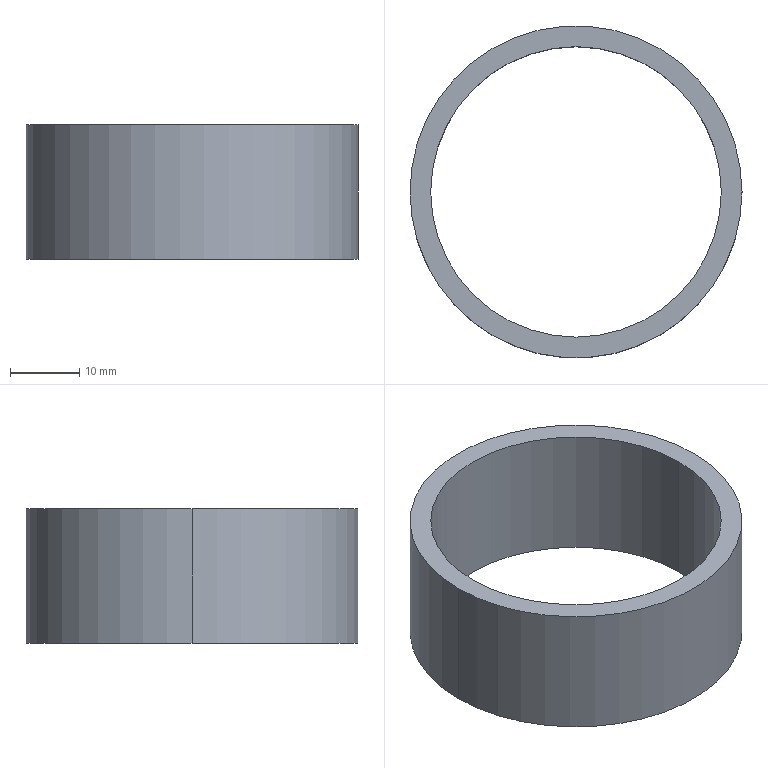Part | STEP file | 04-Spacer 1 | 1 solid | 6 faces | box 48 x 48 x 19.5 mm | volume 8270 mm3 | cylinder 4 | plane 2 | commonest cylinder face diameters 42 x2 48 x2
STEP:
#1=CARTESIAN_POINT('',(0.,0.,0.));
#2=DIRECTION('',(0.,0.,1.));
#3=DIRECTION('',(1.,0.,0.));
#4=AXIS2_PLACEMENT_3D('',#1,#2,#3);
#5=CARTESIAN_POINT('',(-21.,0.,19.5));
#6=VERTEX_POINT('',#5);
#7=CARTESIAN_POINT('',(-21.,0.,0.));
#8=VERTEX_POINT('',#7);
#9=CARTESIAN_POINT('',(-21.,0.,19.5));
#10=DIRECTION('',(0.,0.,-1.));
#11=VECTOR('',#10,1.);
#12=LINE('',#9,#11);
#13=CARTESIAN_POINT('',(0.,0.,19.5));
#14=DIRECTION('',(0.,0.,-1.));
#15=DIRECTION('',(-1.,0.,0.));
#16=AXIS2_PLACEMENT_3D('',#13,#14,#15);
#17=CYLINDRICAL_SURFACE('',#16,21.);
#18=CARTESIAN_POINT('',(6.283,0.));
#19=DIRECTION('',(0.,1.));
#20=VECTOR('',#19,1.);
#21=LINE('',#18,#20);
#22=(GEOMETRIC_REPRESENTATION_CONTEXT(2)PARAMETRIC_REPRESENTATION_CONTEXT()REPRESENTATION_CONTEXT('',''));
#23=DEFINITIONAL_REPRESENTATION('',(#21),#22);
#24=PCURVE('',#17,#23);
#25=CARTESIAN_POINT('',(0.,0.,19.5));
#26=DIRECTION('',(0.,0.,-1.));
#27=DIRECTION('',(-1.,0.,0.));
#28=AXIS2_PLACEMENT_3D('',#25,#26,#27);
#29=CYLINDRICAL_SURFACE('',#28,21.);
#30=CARTESIAN_POINT('',(0.,0.));
#31=DIRECTION('',(0.,1.));
#32=VECTOR('',#31,1.);
#33=LINE('',#30,#32);
#34=(GEOMETRIC_REPRESENTATION_CONTEXT(2)PARAMETRIC_REPRESENTATION_CONTEXT()REPRESENTATION_CONTEXT('',''));
#35=DEFINITIONAL_REPRESENTATION('',(#33),#34);
#36=PCURVE('',#29,#35);
#37=SURFACE_CURVE('',#12,(#24,#36),.PCURVE_S1.);
#38=EDGE_CURVE('',#6,#8,#37,.T.);
#39=ORIENTED_EDGE('',*,*,#38,.T.);
#40=CARTESIAN_POINT('',(21.,0.,0.));
#41=VERTEX_POINT('',#40);
#42=CARTESIAN_POINT('',(0.,0.,0.));
#43=DIRECTION('',(0.,0.,1.));
#44=DIRECTION('',(1.,0.,0.));
#45=AXIS2_PLACEMENT_3D('',#42,#43,#44);
#46=CIRCLE('',#45,21.);
#47=CARTESIAN_POINT('',(9.425,19.5));
#48=DIRECTION('',(-1.,0.));
#49=VECTOR('',#48,1.);
#50=LINE('',#47,#49);
#51=(GEOMETRIC_REPRESENTATION_CONTEXT(2)PARAMETRIC_REPRESENTATION_CONTEXT()REPRESENTATION_CONTEXT('',''));
#52=DEFINITIONAL_REPRESENTATION('',(#50),#51);
#53=PCURVE('',#17,#52);
#54=CARTESIAN_POINT('',(0.,0.,0.));
#55=DIRECTION('',(0.,0.,1.));
#56=DIRECTION('',(1.,0.,0.));
#57=AXIS2_PLACEMENT_3D('',#54,#55,#56);
#58=PLANE('',#57);
#59=CARTESIAN_POINT('',(0.,0.));
#60=DIRECTION('',(1.,0.));
#61=AXIS2_PLACEMENT_2D('',#59,#60);
#62=CIRCLE('',#61,21.);
#63=(GEOMETRIC_REPRESENTATION_CONTEXT(2)PARAMETRIC_REPRESENTATION_CONTEXT()REPRESENTATION_CONTEXT('',''));
#64=DEFINITIONAL_REPRESENTATION('',(#62),#63);
#65=PCURVE('',#58,#64);
#66=SURFACE_CURVE('',#46,(#53,#65),.PCURVE_S1.);
#67=EDGE_CURVE('',#8,#41,#66,.T.);
#68=ORIENTED_EDGE('',*,*,#67,.T.);
#69=CARTESIAN_POINT('',(21.,0.,19.5));
#70=VERTEX_POINT('',#69);
#71=CARTESIAN_POINT('',(21.,0.,19.5));
#72=DIRECTION('',(0.,0.,-1.));
#73=VECTOR('',#72,1.);
#74=LINE('',#71,#73);
#75=CARTESIAN_POINT('',(3.142,0.));
#76=DIRECTION('',(0.,1.));
#77=VECTOR('',#76,1.);
#78=LINE('',#75,#77);
#79=(GEOMETRIC_REPRESENTATION_CONTEXT(2)PARAMETRIC_REPRESENTATION_CONTEXT()REPRESENTATION_CONTEXT('',''));
#80=DEFINITIONAL_REPRESENTATION('',(#78),#79);
#81=PCURVE('',#17,#80);
#82=CARTESIAN_POINT('',(3.142,0.));
#83=DIRECTION('',(0.,1.));
#84=VECTOR('',#83,1.);
#85=LINE('',#82,#84);
#86=(GEOMETRIC_REPRESENTATION_CONTEXT(2)PARAMETRIC_REPRESENTATION_CONTEXT()REPRESENTATION_CONTEXT('',''));
#87=DEFINITIONAL_REPRESENTATION('',(#85),#86);
#88=PCURVE('',#29,#87);
#89=SURFACE_CURVE('',#74,(#81,#88),.PCURVE_S1.);
#90=EDGE_CURVE('',#70,#41,#89,.T.);
#91=ORIENTED_EDGE('',*,*,#90,.F.);
#92=CARTESIAN_POINT('',(0.,0.,19.5));
#93=DIRECTION('',(0.,0.,1.));
#94=DIRECTION('',(1.,0.,0.));
#95=AXIS2_PLACEMENT_3D('',#92,#93,#94);
#96=CIRCLE('',#95,21.);
#97=CARTESIAN_POINT('',(9.425,0.));
#98=DIRECTION('',(-1.,0.));
#99=VECTOR('',#98,1.);
#100=LINE('',#97,#99);
#101=(GEOMETRIC_REPRESENTATION_CONTEXT(2)PARAMETRIC_REPRESENTATION_CONTEXT()REPRESENTATION_CONTEXT('',''));
#102=DEFINITIONAL_REPRESENTATION('',(#100),#101);
#103=PCURVE('',#17,#102);
#104=CARTESIAN_POINT('',(0.,0.,19.5));
#105=DIRECTION('',(0.,0.,1.));
#106=DIRECTION('',(1.,0.,0.));
#107=AXIS2_PLACEMENT_3D('',#104,#105,#106);
#108=PLANE('',#107);
#109=CARTESIAN_POINT('',(0.,0.));
#110=DIRECTION('',(1.,0.));
#111=AXIS2_PLACEMENT_2D('',#109,#110);
#112=CIRCLE('',#111,21.);
#113=(GEOMETRIC_REPRESENTATION_CONTEXT(2)PARAMETRIC_REPRESENTATION_CONTEXT()REPRESENTATION_CONTEXT('',''));
#114=DEFINITIONAL_REPRESENTATION('',(#112),#113);
#115=PCURVE('',#108,#114);
#116=SURFACE_CURVE('',#96,(#103,#115),.PCURVE_S1.);
#117=EDGE_CURVE('',#6,#70,#116,.T.);
#118=ORIENTED_EDGE('',*,*,#117,.F.);
#119=EDGE_LOOP('',(#39,#68,#91,#118));
#120=FACE_BOUND('',#119,.F.);
#121=ADVANCED_FACE('',(#120),#17,.F.);
#122=CARTESIAN_POINT('',(24.,0.,19.5));
#123=VERTEX_POINT('',#122);
#124=CARTESIAN_POINT('',(-24.,0.,19.5));
#125=VERTEX_POINT('',#124);
#126=CARTESIAN_POINT('',(0.,0.,19.5));
#127=DIRECTION('',(0.,0.,1.));
#128=DIRECTION('',(1.,0.,0.));
#129=AXIS2_PLACEMENT_3D('',#126,#127,#128);
#130=CIRCLE('',#129,24.);
#131=CARTESIAN_POINT('',(0.,0.,19.5));
#132=DIRECTION('',(0.,0.,-1.));
#133=DIRECTION('',(-1.,0.,0.));
#134=AXIS2_PLACEMENT_3D('',#131,#132,#133);
#135=CYLINDRICAL_SURFACE('',#134,24.);
#136=CARTESIAN_POINT('',(3.142,0.));
#137=DIRECTION('',(-1.,0.));
#138=VECTOR('',#137,1.);
#139=LINE('',#136,#138);
#140=(GEOMETRIC_REPRESENTATION_CONTEXT(2)PARAMETRIC_REPRESENTATION_CONTEXT()REPRESENTATION_CONTEXT('',''));
#141=DEFINITIONAL_REPRESENTATION('',(#139),#140);
#142=PCURVE('',#135,#141);
#143=CARTESIAN_POINT('',(0.,0.));
#144=DIRECTION('',(1.,0.));
#145=AXIS2_PLACEMENT_2D('',#143,#144);
#146=CIRCLE('',#145,24.);
#147=(GEOMETRIC_REPRESENTATION_CONTEXT(2)PARAMETRIC_REPRESENTATION_CONTEXT()REPRESENTATION_CONTEXT('',''));
#148=DEFINITIONAL_REPRESENTATION('',(#146),#147);
#149=PCURVE('',#108,#148);
#150=SURFACE_CURVE('',#130,(#142,#149),.PCURVE_S1.);
#151=EDGE_CURVE('',#123,#125,#150,.T.);
#152=ORIENTED_EDGE('',*,*,#151,.F.);
#153=CARTESIAN_POINT('',(24.,0.,0.));
#154=VERTEX_POINT('',#153);
#155=CARTESIAN_POINT('',(24.,0.,19.5));
#156=DIRECTION('',(0.,0.,-1.));
#157=VECTOR('',#156,1.);
#158=LINE('',#155,#157);
#159=CARTESIAN_POINT('',(3.142,0.));
#160=DIRECTION('',(0.,1.));
#161=VECTOR('',#160,1.);
#162=LINE('',#159,#161);
#163=(GEOMETRIC_REPRESENTATION_CONTEXT(2)PARAMETRIC_REPRESENTATION_CONTEXT()REPRESENTATION_CONTEXT('',''));
#164=DEFINITIONAL_REPRESENTATION('',(#162),#163);
#165=PCURVE('',#135,#164);
#166=CARTESIAN_POINT('',(0.,0.,19.5));
#167=DIRECTION('',(0.,0.,-1.));
#168=DIRECTION('',(-1.,0.,0.));
#169=AXIS2_PLACEMENT_3D('',#166,#167,#168);
#170=CYLINDRICAL_SURFACE('',#169,24.);
#171=CARTESIAN_POINT('',(3.142,0.));
#172=DIRECTION('',(0.,1.));
#173=VECTOR('',#172,1.);
#174=LINE('',#171,#173);
#175=(GEOMETRIC_REPRESENTATION_CONTEXT(2)PARAMETRIC_REPRESENTATION_CONTEXT()REPRESENTATION_CONTEXT('',''));
#176=DEFINITIONAL_REPRESENTATION('',(#174),#175);
#177=PCURVE('',#170,#176);
#178=SURFACE_CURVE('',#158,(#165,#177),.PCURVE_S1.);
#179=EDGE_CURVE('',#123,#154,#178,.T.);
#180=ORIENTED_EDGE('',*,*,#179,.T.);
#181=CARTESIAN_POINT('',(-24.,0.,0.));
#182=VERTEX_POINT('',#181);
#183=CARTESIAN_POINT('',(0.,0.,0.));
#184=DIRECTION('',(0.,0.,1.));
#185=DIRECTION('',(1.,0.,0.));
#186=AXIS2_PLACEMENT_3D('',#183,#184,#185);
#187=CIRCLE('',#186,24.);
#188=CARTESIAN_POINT('',(3.142,19.5));
#189=DIRECTION('',(-1.,0.));
#190=VECTOR('',#189,1.);
#191=LINE('',#188,#190);
#192=(GEOMETRIC_REPRESENTATION_CONTEXT(2)PARAMETRIC_REPRESENTATION_CONTEXT()REPRESENTATION_CONTEXT('',''));
#193=DEFINITIONAL_REPRESENTATION('',(#191),#192);
#194=PCURVE('',#135,#193);
#195=CARTESIAN_POINT('',(0.,0.));
#196=DIRECTION('',(1.,0.));
#197=AXIS2_PLACEMENT_2D('',#195,#196);
#198=CIRCLE('',#197,24.);
#199=(GEOMETRIC_REPRESENTATION_CONTEXT(2)PARAMETRIC_REPRESENTATION_CONTEXT()REPRESENTATION_CONTEXT('',''));
#200=DEFINITIONAL_REPRESENTATION('',(#198),#199);
#201=PCURVE('',#58,#200);
#202=SURFACE_CURVE('',#187,(#194,#201),.PCURVE_S1.);
#203=EDGE_CURVE('',#154,#182,#202,.T.);
#204=ORIENTED_EDGE('',*,*,#203,.T.);
#205=CARTESIAN_POINT('',(-24.,0.,19.5));
#206=DIRECTION('',(0.,0.,-1.));
#207=VECTOR('',#206,1.);
#208=LINE('',#205,#207);
#209=CARTESIAN_POINT('',(0.,0.));
#210=DIRECTION('',(0.,1.));
#211=VECTOR('',#210,1.);
#212=LINE('',#209,#211);
#213=(GEOMETRIC_REPRESENTATION_CONTEXT(2)PARAMETRIC_REPRESENTATION_CONTEXT()REPRESENTATION_CONTEXT('',''));
#214=DEFINITIONAL_REPRESENTATION('',(#212),#213);
#215=PCURVE('',#135,#214);
#216=CARTESIAN_POINT('',(6.283,0.));
#217=DIRECTION('',(0.,1.));
#218=VECTOR('',#217,1.);
#219=LINE('',#216,#218);
#220=(GEOMETRIC_REPRESENTATION_CONTEXT(2)PARAMETRIC_REPRESENTATION_CONTEXT()REPRESENTATION_CONTEXT('',''));
#221=DEFINITIONAL_REPRESENTATION('',(#219),#220);
#222=PCURVE('',#170,#221);
#223=SURFACE_CURVE('',#208,(#215,#222),.PCURVE_S1.);
#224=EDGE_CURVE('',#125,#182,#223,.T.);
#225=ORIENTED_EDGE('',*,*,#224,.F.);
#226=EDGE_LOOP('',(#152,#180,#204,#225));
#227=FACE_BOUND('',#226,.T.);
#228=ADVANCED_FACE('',(#227),#135,.T.);
#229=CARTESIAN_POINT('',(0.,0.,19.5));
#230=DIRECTION('',(0.,0.,1.));
#231=DIRECTION('',(1.,0.,0.));
#232=AXIS2_PLACEMENT_3D('',#229,#230,#231);
#233=CIRCLE('',#232,24.);
#234=CARTESIAN_POINT('',(0.,0.));
#235=DIRECTION('',(1.,0.));
#236=AXIS2_PLACEMENT_2D('',#234,#235);
#237=CIRCLE('',#236,24.);
#238=(GEOMETRIC_REPRESENTATION_CONTEXT(2)PARAMETRIC_REPRESENTATION_CONTEXT()REPRESENTATION_CONTEXT('',''));
#239=DEFINITIONAL_REPRESENTATION('',(#237),#238);
#240=PCURVE('',#108,#239);
#241=CARTESIAN_POINT('',(9.425,0.));
#242=DIRECTION('',(-1.,0.));
#243=VECTOR('',#242,1.);
#244=LINE('',#241,#243);
#245=(GEOMETRIC_REPRESENTATION_CONTEXT(2)PARAMETRIC_REPRESENTATION_CONTEXT()REPRESENTATION_CONTEXT('',''));
#246=DEFINITIONAL_REPRESENTATION('',(#244),#245);
#247=PCURVE('',#170,#246);
#248=SURFACE_CURVE('',#233,(#240,#247),.PCURVE_S1.);
#249=EDGE_CURVE('',#125,#123,#248,.T.);
#250=ORIENTED_EDGE('',*,*,#249,.T.);
#251=ORIENTED_EDGE('',*,*,#151,.T.);
#252=EDGE_LOOP('',(#250,#251));
#253=FACE_BOUND('',#252,.T.);
#254=ORIENTED_EDGE('',*,*,#117,.F.);
#255=CARTESIAN_POINT('',(0.,0.,19.5));
#256=DIRECTION('',(0.,0.,1.));
#257=DIRECTION('',(1.,0.,0.));
#258=AXIS2_PLACEMENT_3D('',#255,#256,#257);
#259=CIRCLE('',#258,21.);
#260=CARTESIAN_POINT('',(0.,0.));
#261=DIRECTION('',(1.,0.));
#262=AXIS2_PLACEMENT_2D('',#260,#261);
#263=CIRCLE('',#262,21.);
#264=(GEOMETRIC_REPRESENTATION_CONTEXT(2)PARAMETRIC_REPRESENTATION_CONTEXT()REPRESENTATION_CONTEXT('',''));
#265=DEFINITIONAL_REPRESENTATION('',(#263),#264);
#266=PCURVE('',#108,#265);
#267=CARTESIAN_POINT('',(3.142,0.));
#268=DIRECTION('',(-1.,0.));
#269=VECTOR('',#268,1.);
#270=LINE('',#267,#269);
#271=(GEOMETRIC_REPRESENTATION_CONTEXT(2)PARAMETRIC_REPRESENTATION_CONTEXT()REPRESENTATION_CONTEXT('',''));
#272=DEFINITIONAL_REPRESENTATION('',(#270),#271);
#273=PCURVE('',#29,#272);
#274=SURFACE_CURVE('',#259,(#266,#273),.PCURVE_S1.);
#275=EDGE_CURVE('',#70,#6,#274,.T.);
#276=ORIENTED_EDGE('',*,*,#275,.F.);
#277=EDGE_LOOP('',(#254,#276));
#278=FACE_BOUND('',#277,.T.);
#279=ADVANCED_FACE('',(#253,#278),#108,.T.);
#280=CARTESIAN_POINT('',(0.,0.,0.));
#281=DIRECTION('',(0.,0.,1.));
#282=DIRECTION('',(1.,0.,0.));
#283=AXIS2_PLACEMENT_3D('',#280,#281,#282);
#284=CIRCLE('',#283,24.);
#285=CARTESIAN_POINT('',(0.,0.));
#286=DIRECTION('',(1.,0.));
#287=AXIS2_PLACEMENT_2D('',#285,#286);
#288=CIRCLE('',#287,24.);
#289=(GEOMETRIC_REPRESENTATION_CONTEXT(2)PARAMETRIC_REPRESENTATION_CONTEXT()REPRESENTATION_CONTEXT('',''));
#290=DEFINITIONAL_REPRESENTATION('',(#288),#289);
#291=PCURVE('',#58,#290);
#292=CARTESIAN_POINT('',(9.425,19.5));
#293=DIRECTION('',(-1.,0.));
#294=VECTOR('',#293,1.);
#295=LINE('',#292,#294);
#296=(GEOMETRIC_REPRESENTATION_CONTEXT(2)PARAMETRIC_REPRESENTATION_CONTEXT()REPRESENTATION_CONTEXT('',''));
#297=DEFINITIONAL_REPRESENTATION('',(#295),#296);
#298=PCURVE('',#170,#297);
#299=SURFACE_CURVE('',#284,(#291,#298),.PCURVE_S1.);
#300=EDGE_CURVE('',#182,#154,#299,.T.);
#301=ORIENTED_EDGE('',*,*,#300,.F.);
#302=ORIENTED_EDGE('',*,*,#203,.F.);
#303=EDGE_LOOP('',(#301,#302));
#304=FACE_BOUND('',#303,.T.);
#305=ORIENTED_EDGE('',*,*,#67,.T.);
#306=CARTESIAN_POINT('',(0.,0.,0.));
#307=DIRECTION('',(0.,0.,1.));
#308=DIRECTION('',(1.,0.,0.));
#309=AXIS2_PLACEMENT_3D('',#306,#307,#308);
#310=CIRCLE('',#309,21.);
#311=CARTESIAN_POINT('',(0.,0.));
#312=DIRECTION('',(1.,0.));
#313=AXIS2_PLACEMENT_2D('',#311,#312);
#314=CIRCLE('',#313,21.);
#315=(GEOMETRIC_REPRESENTATION_CONTEXT(2)PARAMETRIC_REPRESENTATION_CONTEXT()REPRESENTATION_CONTEXT('',''));
#316=DEFINITIONAL_REPRESENTATION('',(#314),#315);
#317=PCURVE('',#58,#316);
#318=CARTESIAN_POINT('',(3.142,19.5));
#319=DIRECTION('',(-1.,0.));
#320=VECTOR('',#319,1.);
#321=LINE('',#318,#320);
#322=(GEOMETRIC_REPRESENTATION_CONTEXT(2)PARAMETRIC_REPRESENTATION_CONTEXT()REPRESENTATION_CONTEXT('',''));
#323=DEFINITIONAL_REPRESENTATION('',(#321),#322);
#324=PCURVE('',#29,#323);
#325=SURFACE_CURVE('',#310,(#317,#324),.PCURVE_S1.);
#326=EDGE_CURVE('',#41,#8,#325,.T.);
#327=ORIENTED_EDGE('',*,*,#326,.T.);
#328=EDGE_LOOP('',(#305,#327));
#329=FACE_BOUND('',#328,.T.);
#330=ADVANCED_FACE('',(#304,#329),#58,.F.);
#331=ORIENTED_EDGE('',*,*,#179,.F.);
#332=ORIENTED_EDGE('',*,*,#249,.F.);
#333=ORIENTED_EDGE('',*,*,#224,.T.);
#334=ORIENTED_EDGE('',*,*,#300,.T.);
#335=EDGE_LOOP('',(#331,#332,#333,#334));
#336=FACE_BOUND('',#335,.T.);
#337=ADVANCED_FACE('',(#336),#170,.T.);
#338=ORIENTED_EDGE('',*,*,#326,.T.);
#339=ORIENTED_EDGE('',*,*,#38,.F.);
#340=ORIENTED_EDGE('',*,*,#275,.F.);
#341=ORIENTED_EDGE('',*,*,#90,.T.);
#342=EDGE_LOOP('',(#338,#339,#340,#341));
#343=FACE_BOUND('',#342,.F.);
#344=ADVANCED_FACE('',(#343),#29,.F.);
#345=CLOSED_SHELL('',(#121,#228,#279,#330,#337,#344));
#346=MANIFOLD_SOLID_BREP('',#345);
#347=(LENGTH_UNIT()NAMED_UNIT(*)SI_UNIT(.MILLI.,.METRE.));
#348=UNCERTAINTY_MEASURE_WITH_UNIT(LENGTH_MEASURE(0.0000001),#347,'','');
#349=(NAMED_UNIT(*)PLANE_ANGLE_UNIT()SI_UNIT($,.RADIAN.));
#350=(NAMED_UNIT(*)SI_UNIT($,.STERADIAN.)SOLID_ANGLE_UNIT());
#351=(GEOMETRIC_REPRESENTATION_CONTEXT(3)GLOBAL_UNCERTAINTY_ASSIGNED_CONTEXT((#348))GLOBAL_UNIT_ASSIGNED_CONTEXT((#347,#349,#350))REPRESENTATION_CONTEXT('',''));
#352=ADVANCED_BREP_SHAPE_REPRESENTATION('',(#4,#346),#351);